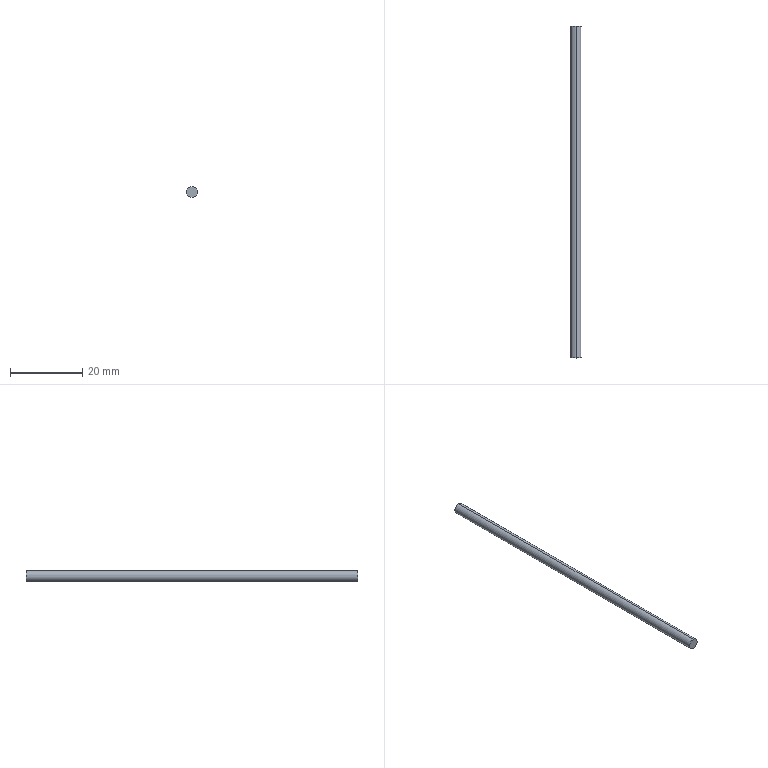Part | SolidWorks | features Revolution 1 | 1 solid | 4 faces | box 3 x 92 x 3 mm | volume 650.31 mm3 | cylinder 2 | plane 2 | commonest cylinder face diameters 3 x2
STEP:
#1=CARTESIAN_POINT('',(0.,92.,-1.5));
#2=VERTEX_POINT('',#1);
#3=CARTESIAN_POINT('',(0.,92.,1.5));
#4=VERTEX_POINT('',#3);
#5=CARTESIAN_POINT('',(0.,92.,0.));
#6=DIRECTION('',(0.,-1.,0.));
#7=DIRECTION('',(0.,0.,-1.));
#8=AXIS2_PLACEMENT_3D('',#5,#6,#7);
#9=CIRCLE('',#8,1.5);
#10=EDGE_CURVE('',#2,#4,#9,.T.);
#11=ORIENTED_EDGE('',*,*,#10,.T.);
#12=CARTESIAN_POINT('',(0.,0.,1.5));
#13=VERTEX_POINT('',#12);
#14=CARTESIAN_POINT('',(0.,0.,1.5));
#15=DIRECTION('',(0.,-1.,0.));
#16=VECTOR('',#15,1000.);
#17=LINE('',#14,#16);
#18=EDGE_CURVE('',#4,#13,#17,.T.);
#19=ORIENTED_EDGE('',*,*,#18,.T.);
#20=CARTESIAN_POINT('',(0.,0.,-1.5));
#21=VERTEX_POINT('',#20);
#22=CARTESIAN_POINT('',(0.,0.,0.));
#23=DIRECTION('',(0.,-1.,0.));
#24=DIRECTION('',(0.,0.,-1.));
#25=AXIS2_PLACEMENT_3D('',#22,#23,#24);
#26=CIRCLE('',#25,1.5);
#27=EDGE_CURVE('',#21,#13,#26,.T.);
#28=ORIENTED_EDGE('',*,*,#27,.F.);
#29=CARTESIAN_POINT('',(0.,0.,-1.5));
#30=DIRECTION('',(0.,-1.,0.));
#31=VECTOR('',#30,1000.);
#32=LINE('',#29,#31);
#33=EDGE_CURVE('',#2,#21,#32,.T.);
#34=ORIENTED_EDGE('',*,*,#33,.F.);
#35=EDGE_LOOP('',(#11,#19,#28,#34));
#36=FACE_OUTER_BOUND('',#35,.T.);
#37=CARTESIAN_POINT('',(0.,0.,0.));
#38=DIRECTION('',(0.,-1.,0.));
#39=DIRECTION('',(0.,0.,-1.));
#40=AXIS2_PLACEMENT_3D('',#37,#38,#39);
#41=CYLINDRICAL_SURFACE('',#40,1.5);
#42=ADVANCED_FACE('',(#36),#41,.T.);
#43=ORIENTED_EDGE('',*,*,#10,.F.);
#44=CARTESIAN_POINT('',(0.,92.,0.));
#45=DIRECTION('',(0.,-1.,0.));
#46=DIRECTION('',(0.,0.,-1.));
#47=AXIS2_PLACEMENT_3D('',#44,#45,#46);
#48=CIRCLE('',#47,1.5);
#49=EDGE_CURVE('',#4,#2,#48,.T.);
#50=ORIENTED_EDGE('',*,*,#49,.F.);
#51=EDGE_LOOP('',(#43,#50));
#52=FACE_OUTER_BOUND('',#51,.T.);
#53=CARTESIAN_POINT('',(1.5,92.,0.));
#54=DIRECTION('',(0.,1.,0.));
#55=DIRECTION('',(0.,0.,1.));
#56=AXIS2_PLACEMENT_3D('',#53,#54,#55);
#57=PLANE('',#56);
#58=ADVANCED_FACE('',(#52),#57,.T.);
#59=ORIENTED_EDGE('',*,*,#18,.F.);
#60=ORIENTED_EDGE('',*,*,#49,.T.);
#61=ORIENTED_EDGE('',*,*,#33,.T.);
#62=CARTESIAN_POINT('',(0.,0.,0.));
#63=DIRECTION('',(0.,-1.,0.));
#64=DIRECTION('',(0.,0.,-1.));
#65=AXIS2_PLACEMENT_3D('',#62,#63,#64);
#66=CIRCLE('',#65,1.5);
#67=EDGE_CURVE('',#13,#21,#66,.T.);
#68=ORIENTED_EDGE('',*,*,#67,.F.);
#69=EDGE_LOOP('',(#59,#60,#61,#68));
#70=FACE_OUTER_BOUND('',#69,.T.);
#71=CARTESIAN_POINT('',(0.,0.,0.));
#72=DIRECTION('',(0.,-1.,0.));
#73=DIRECTION('',(0.,0.,-1.));
#74=AXIS2_PLACEMENT_3D('',#71,#72,#73);
#75=CYLINDRICAL_SURFACE('',#74,1.5);
#76=ADVANCED_FACE('',(#70),#75,.T.);
#77=ORIENTED_EDGE('',*,*,#27,.T.);
#78=ORIENTED_EDGE('',*,*,#67,.T.);
#79=EDGE_LOOP('',(#77,#78));
#80=FACE_OUTER_BOUND('',#79,.T.);
#81=CARTESIAN_POINT('',(0.,0.,0.));
#82=DIRECTION('',(0.,-1.,0.));
#83=DIRECTION('',(0.,0.,-1.));
#84=AXIS2_PLACEMENT_3D('',#81,#82,#83);
#85=PLANE('',#84);
#86=ADVANCED_FACE('',(#80),#85,.T.);
#87=CLOSED_SHELL('',(#42,#58,#76,#86));
#88=MANIFOLD_SOLID_BREP('',#87);
#89=CARTESIAN_POINT('',(0.,0.,0.));
#90=DIRECTION('',(0.,0.,1.));
#91=DIRECTION('',(1.,0.,0.));
#92=AXIS2_PLACEMENT_3D('',#89,#90,#91);
#93=(LENGTH_UNIT()NAMED_UNIT(*)SI_UNIT(.MILLI.,.METRE.));
#94=UNCERTAINTY_MEASURE_WITH_UNIT(LENGTH_MEASURE(0.00001),#93,'','');
#95=(NAMED_UNIT(*)PLANE_ANGLE_UNIT()SI_UNIT($,.RADIAN.));
#96=(NAMED_UNIT(*)SI_UNIT($,.STERADIAN.)SOLID_ANGLE_UNIT());
#97=(GEOMETRIC_REPRESENTATION_CONTEXT(3)GLOBAL_UNCERTAINTY_ASSIGNED_CONTEXT((#94))GLOBAL_UNIT_ASSIGNED_CONTEXT((#93,#95,#96))REPRESENTATION_CONTEXT('',''));
#98=ADVANCED_BREP_SHAPE_REPRESENTATION('',(#88,#92),#97);